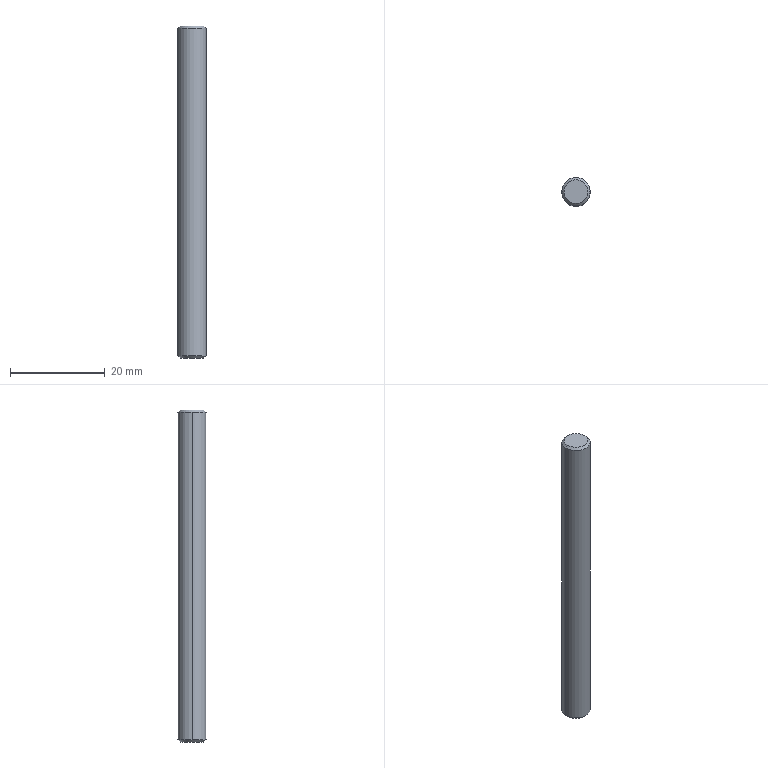Part | SolidWorks | features Chamfer 1, Extrusion 1 | 1 solid | 8 faces | box 6 x 6 x 70 mm | volume 1975 mm3 | cone 4 | cylinder 2 | plane 2 | commonest cylinder face diameters 6 x2
STEP:
#1=CARTESIAN_POINT('',(83.5,-185.452,0.));
#2=VERTEX_POINT('',#1);
#3=CARTESIAN_POINT('',(78.5,-185.452,0.));
#4=VERTEX_POINT('',#3);
#5=CARTESIAN_POINT('',(81.,-185.452,0.));
#6=DIRECTION('',(0.,0.,1.));
#7=DIRECTION('',(1.,0.,0.));
#8=AXIS2_PLACEMENT_3D('',#5,#6,#7);
#9=CIRCLE('',#8,2.5);
#10=EDGE_CURVE('',#2,#4,#9,.T.);
#11=ORIENTED_EDGE('',*,*,#10,.F.);
#12=CARTESIAN_POINT('',(84.,-185.452,-0.5));
#13=VERTEX_POINT('',#12);
#14=CARTESIAN_POINT('',(83.5,-185.452,0.));
#15=DIRECTION('',(0.7071,0.,-0.7071));
#16=VECTOR('',#15,1000.);
#17=LINE('',#14,#16);
#18=EDGE_CURVE('',#2,#13,#17,.T.);
#19=ORIENTED_EDGE('',*,*,#18,.T.);
#20=CARTESIAN_POINT('',(78.,-185.452,-0.5));
#21=VERTEX_POINT('',#20);
#22=CARTESIAN_POINT('',(81.,-185.452,-0.5));
#23=DIRECTION('',(0.,0.,-1.));
#24=DIRECTION('',(1.,0.,0.));
#25=AXIS2_PLACEMENT_3D('',#22,#23,#24);
#26=CIRCLE('',#25,3.);
#27=EDGE_CURVE('',#21,#13,#26,.T.);
#28=ORIENTED_EDGE('',*,*,#27,.F.);
#29=CARTESIAN_POINT('',(78.5,-185.452,0.));
#30=DIRECTION('',(-0.7071,0.,-0.7071));
#31=VECTOR('',#30,1000.);
#32=LINE('',#29,#31);
#33=EDGE_CURVE('',#4,#21,#32,.T.);
#34=ORIENTED_EDGE('',*,*,#33,.F.);
#35=EDGE_LOOP('',(#11,#19,#28,#34));
#36=FACE_OUTER_BOUND('',#35,.T.);
#37=CARTESIAN_POINT('',(81.,-185.452,0.));
#38=DIRECTION('',(0.,0.,-1.));
#39=DIRECTION('',(-1.,0.,0.));
#40=AXIS2_PLACEMENT_3D('',#37,#38,#39);
#41=CONICAL_SURFACE('',#40,2.5,0.7854);
#42=ADVANCED_FACE('',(#36),#41,.T.);
#43=CARTESIAN_POINT('',(78.5,-185.452,-70.));
#44=VERTEX_POINT('',#43);
#45=CARTESIAN_POINT('',(83.5,-185.452,-70.));
#46=VERTEX_POINT('',#45);
#47=CARTESIAN_POINT('',(81.,-185.452,-70.));
#48=DIRECTION('',(0.,0.,-1.));
#49=DIRECTION('',(1.,0.,0.));
#50=AXIS2_PLACEMENT_3D('',#47,#48,#49);
#51=CIRCLE('',#50,2.5);
#52=EDGE_CURVE('',#44,#46,#51,.T.);
#53=ORIENTED_EDGE('',*,*,#52,.F.);
#54=CARTESIAN_POINT('',(78.,-185.452,-69.5));
#55=VERTEX_POINT('',#54);
#56=CARTESIAN_POINT('',(78.,-185.452,-69.5));
#57=DIRECTION('',(-0.7071,0.,0.7071));
#58=VECTOR('',#57,1000.);
#59=LINE('',#56,#58);
#60=EDGE_CURVE('',#44,#55,#59,.T.);
#61=ORIENTED_EDGE('',*,*,#60,.T.);
#62=CARTESIAN_POINT('',(84.,-185.452,-69.5));
#63=VERTEX_POINT('',#62);
#64=CARTESIAN_POINT('',(81.,-185.452,-69.5));
#65=DIRECTION('',(0.,0.,1.));
#66=DIRECTION('',(1.,0.,0.));
#67=AXIS2_PLACEMENT_3D('',#64,#65,#66);
#68=CIRCLE('',#67,3.);
#69=EDGE_CURVE('',#63,#55,#68,.T.);
#70=ORIENTED_EDGE('',*,*,#69,.F.);
#71=CARTESIAN_POINT('',(84.,-185.452,-69.5));
#72=DIRECTION('',(0.7071,0.,0.7071));
#73=VECTOR('',#72,1000.);
#74=LINE('',#71,#73);
#75=EDGE_CURVE('',#46,#63,#74,.T.);
#76=ORIENTED_EDGE('',*,*,#75,.F.);
#77=EDGE_LOOP('',(#53,#61,#70,#76));
#78=FACE_OUTER_BOUND('',#77,.T.);
#79=CARTESIAN_POINT('',(81.,-185.452,-69.5));
#80=DIRECTION('',(0.,0.,1.));
#81=DIRECTION('',(1.,0.,0.));
#82=AXIS2_PLACEMENT_3D('',#79,#80,#81);
#83=CONICAL_SURFACE('',#82,3.,0.7854);
#84=ADVANCED_FACE('',(#78),#83,.T.);
#85=ORIENTED_EDGE('',*,*,#69,.T.);
#86=CARTESIAN_POINT('',(78.,-185.452,-70.));
#87=DIRECTION('',(0.,0.,1.));
#88=VECTOR('',#87,1000.);
#89=LINE('',#86,#88);
#90=EDGE_CURVE('',#55,#21,#89,.T.);
#91=ORIENTED_EDGE('',*,*,#90,.T.);
#92=ORIENTED_EDGE('',*,*,#27,.T.);
#93=CARTESIAN_POINT('',(84.,-185.452,-70.));
#94=DIRECTION('',(0.,0.,1.));
#95=VECTOR('',#94,1000.);
#96=LINE('',#93,#95);
#97=EDGE_CURVE('',#63,#13,#96,.T.);
#98=ORIENTED_EDGE('',*,*,#97,.F.);
#99=EDGE_LOOP('',(#85,#91,#92,#98));
#100=FACE_OUTER_BOUND('',#99,.T.);
#101=CARTESIAN_POINT('',(81.,-185.452,-70.));
#102=DIRECTION('',(0.,0.,1.));
#103=DIRECTION('',(1.,0.,0.));
#104=AXIS2_PLACEMENT_3D('',#101,#102,#103);
#105=CYLINDRICAL_SURFACE('',#104,3.);
#106=ADVANCED_FACE('',(#100),#105,.T.);
#107=ORIENTED_EDGE('',*,*,#90,.F.);
#108=CARTESIAN_POINT('',(81.,-185.452,-69.5));
#109=DIRECTION('',(0.,0.,1.));
#110=DIRECTION('',(1.,0.,0.));
#111=AXIS2_PLACEMENT_3D('',#108,#109,#110);
#112=CIRCLE('',#111,3.);
#113=EDGE_CURVE('',#55,#63,#112,.T.);
#114=ORIENTED_EDGE('',*,*,#113,.T.);
#115=ORIENTED_EDGE('',*,*,#97,.T.);
#116=CARTESIAN_POINT('',(81.,-185.452,-0.5));
#117=DIRECTION('',(0.,0.,-1.));
#118=DIRECTION('',(1.,0.,0.));
#119=AXIS2_PLACEMENT_3D('',#116,#117,#118);
#120=CIRCLE('',#119,3.);
#121=EDGE_CURVE('',#13,#21,#120,.T.);
#122=ORIENTED_EDGE('',*,*,#121,.T.);
#123=EDGE_LOOP('',(#107,#114,#115,#122));
#124=FACE_OUTER_BOUND('',#123,.T.);
#125=CARTESIAN_POINT('',(81.,-185.452,-70.));
#126=DIRECTION('',(0.,0.,1.));
#127=DIRECTION('',(1.,0.,0.));
#128=AXIS2_PLACEMENT_3D('',#125,#126,#127);
#129=CYLINDRICAL_SURFACE('',#128,3.);
#130=ADVANCED_FACE('',(#124),#129,.T.);
#131=CARTESIAN_POINT('',(81.,-185.452,-70.));
#132=DIRECTION('',(0.,0.,-1.));
#133=DIRECTION('',(1.,0.,0.));
#134=AXIS2_PLACEMENT_3D('',#131,#132,#133);
#135=CIRCLE('',#134,2.5);
#136=EDGE_CURVE('',#46,#44,#135,.T.);
#137=ORIENTED_EDGE('',*,*,#136,.T.);
#138=ORIENTED_EDGE('',*,*,#52,.T.);
#139=EDGE_LOOP('',(#137,#138));
#140=FACE_OUTER_BOUND('',#139,.T.);
#141=CARTESIAN_POINT('',(81.,-185.452,-70.));
#142=DIRECTION('',(0.,0.,1.));
#143=DIRECTION('',(1.,0.,0.));
#144=AXIS2_PLACEMENT_3D('',#141,#142,#143);
#145=PLANE('',#144);
#146=ADVANCED_FACE('',(#140),#145,.F.);
#147=CARTESIAN_POINT('',(81.,-185.452,0.));
#148=DIRECTION('',(0.,0.,1.));
#149=DIRECTION('',(1.,0.,0.));
#150=AXIS2_PLACEMENT_3D('',#147,#148,#149);
#151=CIRCLE('',#150,2.5);
#152=EDGE_CURVE('',#4,#2,#151,.T.);
#153=ORIENTED_EDGE('',*,*,#152,.T.);
#154=ORIENTED_EDGE('',*,*,#10,.T.);
#155=EDGE_LOOP('',(#153,#154));
#156=FACE_OUTER_BOUND('',#155,.T.);
#157=CARTESIAN_POINT('',(81.,-185.452,0.));
#158=DIRECTION('',(0.,0.,1.));
#159=DIRECTION('',(1.,0.,0.));
#160=AXIS2_PLACEMENT_3D('',#157,#158,#159);
#161=PLANE('',#160);
#162=ADVANCED_FACE('',(#156),#161,.T.);
#163=ORIENTED_EDGE('',*,*,#60,.F.);
#164=ORIENTED_EDGE('',*,*,#136,.F.);
#165=ORIENTED_EDGE('',*,*,#75,.T.);
#166=ORIENTED_EDGE('',*,*,#113,.F.);
#167=EDGE_LOOP('',(#163,#164,#165,#166));
#168=FACE_OUTER_BOUND('',#167,.T.);
#169=CARTESIAN_POINT('',(81.,-185.452,-69.5));
#170=DIRECTION('',(0.,0.,1.));
#171=DIRECTION('',(1.,0.,0.));
#172=AXIS2_PLACEMENT_3D('',#169,#170,#171);
#173=CONICAL_SURFACE('',#172,3.,0.7854);
#174=ADVANCED_FACE('',(#168),#173,.T.);
#175=ORIENTED_EDGE('',*,*,#18,.F.);
#176=ORIENTED_EDGE('',*,*,#152,.F.);
#177=ORIENTED_EDGE('',*,*,#33,.T.);
#178=ORIENTED_EDGE('',*,*,#121,.F.);
#179=EDGE_LOOP('',(#175,#176,#177,#178));
#180=FACE_OUTER_BOUND('',#179,.T.);
#181=CARTESIAN_POINT('',(81.,-185.452,0.));
#182=DIRECTION('',(0.,0.,-1.));
#183=DIRECTION('',(-1.,0.,0.));
#184=AXIS2_PLACEMENT_3D('',#181,#182,#183);
#185=CONICAL_SURFACE('',#184,2.5,0.7854);
#186=ADVANCED_FACE('',(#180),#185,.T.);
#187=CLOSED_SHELL('',(#42,#84,#106,#130,#146,#162,#174,#186));
#188=MANIFOLD_SOLID_BREP('',#187);
#189=CARTESIAN_POINT('',(0.,0.,0.));
#190=DIRECTION('',(0.,0.,1.));
#191=DIRECTION('',(1.,0.,0.));
#192=AXIS2_PLACEMENT_3D('',#189,#190,#191);
#193=(LENGTH_UNIT()NAMED_UNIT(*)SI_UNIT(.MILLI.,.METRE.));
#194=UNCERTAINTY_MEASURE_WITH_UNIT(LENGTH_MEASURE(0.00001),#193,'','');
#195=(NAMED_UNIT(*)PLANE_ANGLE_UNIT()SI_UNIT($,.RADIAN.));
#196=(NAMED_UNIT(*)SI_UNIT($,.STERADIAN.)SOLID_ANGLE_UNIT());
#197=(GEOMETRIC_REPRESENTATION_CONTEXT(3)GLOBAL_UNCERTAINTY_ASSIGNED_CONTEXT((#194))GLOBAL_UNIT_ASSIGNED_CONTEXT((#193,#195,#196))REPRESENTATION_CONTEXT('',''));
#198=ADVANCED_BREP_SHAPE_REPRESENTATION('',(#188,#192),#197);